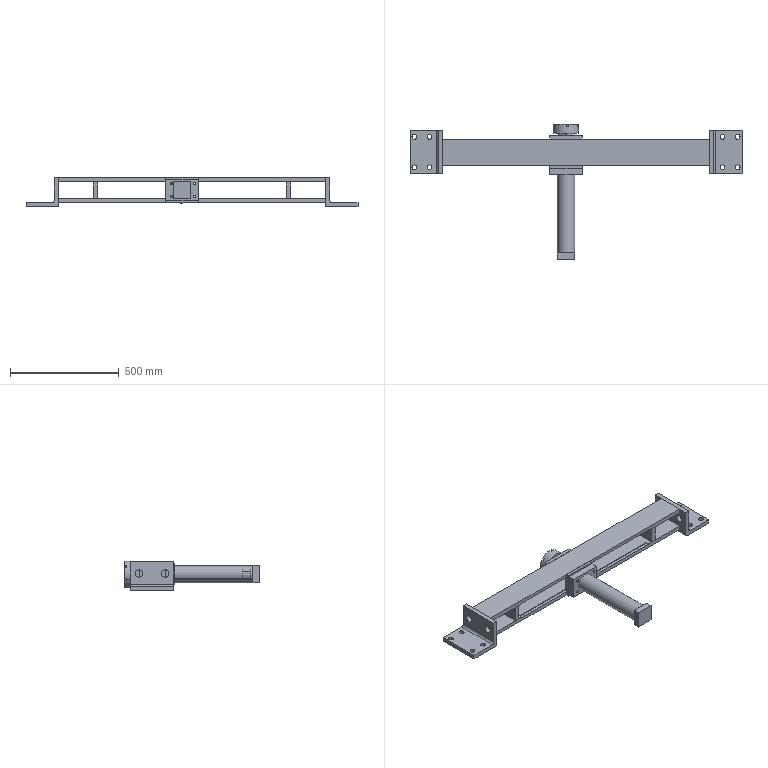Part | SolidWorks | 15 solids | 237 faces | box 1530 x 622 x 137.5 mm | volume 11760878 mm3 | plane 129 | cylinder 98 | cone 10 | commonest cylinder face diameters 10.2 x16 22 x16 12 x8 20 x8 35 x8 80 x8